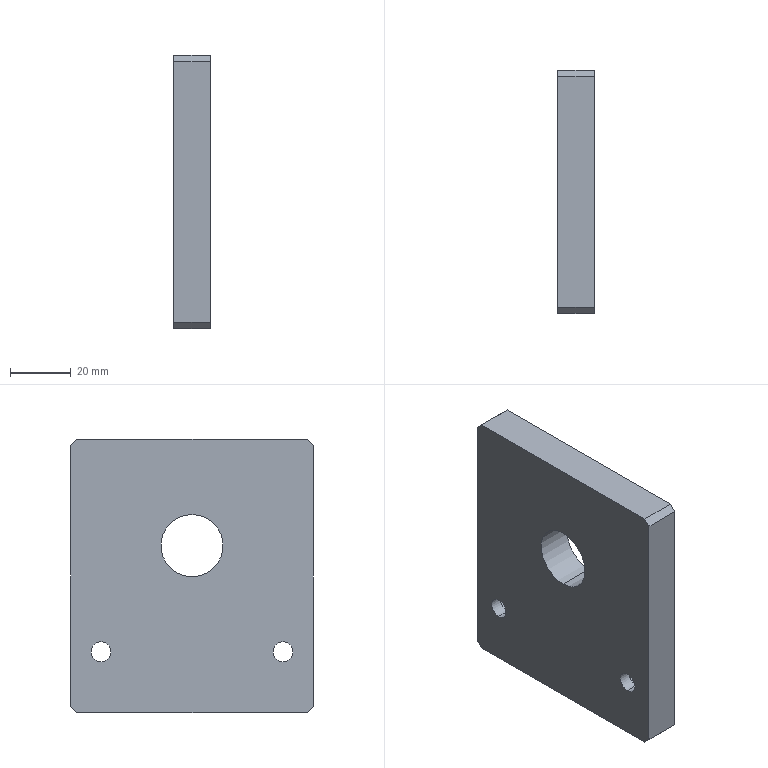Part | SolidWorks | features BaseBody 1 | 1 solid | 22 faces | box 12 x 80 x 90 mm | volume 80549 mm3 | plane 12 | cylinder 10 | commonest cylinder face diameters 6.6 x4 11 x4 20.5 x2
STEP:
#1=CARTESIAN_POINT('',(12.,40.,-45.25));
#2=VERTEX_POINT('',#1);
#3=CARTESIAN_POINT('',(12.,40.,-24.75));
#4=VERTEX_POINT('',#3);
#5=CARTESIAN_POINT('',(12.,40.,-35.));
#6=DIRECTION('',(-1.,0.,0.));
#7=DIRECTION('',(0.,0.,1.));
#8=AXIS2_PLACEMENT_3D('',#5,#6,#7);
#9=CIRCLE('',#8,10.25);
#10=EDGE_CURVE('',#2,#4,#9,.T.);
#11=ORIENTED_EDGE('',*,*,#10,.F.);
#12=CARTESIAN_POINT('',(0.,40.,-45.25));
#13=VERTEX_POINT('',#12);
#14=CARTESIAN_POINT('',(0.,40.,-45.25));
#15=DIRECTION('',(-1.,0.,0.));
#16=VECTOR('',#15,1000.);
#17=LINE('',#14,#16);
#18=EDGE_CURVE('',#2,#13,#17,.T.);
#19=ORIENTED_EDGE('',*,*,#18,.T.);
#20=CARTESIAN_POINT('',(0.,40.,-24.75));
#21=VERTEX_POINT('',#20);
#22=CARTESIAN_POINT('',(0.,40.,-35.));
#23=DIRECTION('',(1.,0.,0.));
#24=DIRECTION('',(0.,0.,1.));
#25=AXIS2_PLACEMENT_3D('',#22,#23,#24);
#26=CIRCLE('',#25,10.25);
#27=EDGE_CURVE('',#21,#13,#26,.T.);
#28=ORIENTED_EDGE('',*,*,#27,.F.);
#29=CARTESIAN_POINT('',(0.,40.,-24.75));
#30=DIRECTION('',(-1.,0.,0.));
#31=VECTOR('',#30,1000.);
#32=LINE('',#29,#31);
#33=EDGE_CURVE('',#4,#21,#32,.T.);
#34=ORIENTED_EDGE('',*,*,#33,.F.);
#35=EDGE_LOOP('',(#11,#19,#28,#34));
#36=FACE_OUTER_BOUND('',#35,.T.);
#37=CARTESIAN_POINT('',(0.,40.,-35.));
#38=DIRECTION('',(-1.,0.,0.));
#39=DIRECTION('',(0.,0.,1.));
#40=AXIS2_PLACEMENT_3D('',#37,#38,#39);
#41=CYLINDRICAL_SURFACE('',#40,10.25);
#42=ADVANCED_FACE('',(#36),#41,.F.);
#43=CARTESIAN_POINT('',(0.,10.,-66.7));
#44=VERTEX_POINT('',#43);
#45=CARTESIAN_POINT('',(0.,10.,-73.3));
#46=VERTEX_POINT('',#45);
#47=CARTESIAN_POINT('',(0.,10.,-70.));
#48=DIRECTION('',(1.,0.,0.));
#49=DIRECTION('',(0.,0.,-1.));
#50=AXIS2_PLACEMENT_3D('',#47,#48,#49);
#51=CIRCLE('',#50,3.3);
#52=EDGE_CURVE('',#44,#46,#51,.T.);
#53=ORIENTED_EDGE('',*,*,#52,.F.);
#54=CARTESIAN_POINT('',(4.,10.,-66.7));
#55=VERTEX_POINT('',#54);
#56=CARTESIAN_POINT('',(12.,10.,-66.7));
#57=DIRECTION('',(1.,0.,0.));
#58=VECTOR('',#57,1000.);
#59=LINE('',#56,#58);
#60=EDGE_CURVE('',#44,#55,#59,.T.);
#61=ORIENTED_EDGE('',*,*,#60,.T.);
#62=CARTESIAN_POINT('',(4.,10.,-73.3));
#63=VERTEX_POINT('',#62);
#64=CARTESIAN_POINT('',(4.,10.,-70.));
#65=DIRECTION('',(-1.,0.,0.));
#66=DIRECTION('',(0.,0.,-1.));
#67=AXIS2_PLACEMENT_3D('',#64,#65,#66);
#68=CIRCLE('',#67,3.3);
#69=EDGE_CURVE('',#63,#55,#68,.T.);
#70=ORIENTED_EDGE('',*,*,#69,.F.);
#71=CARTESIAN_POINT('',(12.,10.,-73.3));
#72=DIRECTION('',(1.,0.,0.));
#73=VECTOR('',#72,1000.);
#74=LINE('',#71,#73);
#75=EDGE_CURVE('',#46,#63,#74,.T.);
#76=ORIENTED_EDGE('',*,*,#75,.F.);
#77=EDGE_LOOP('',(#53,#61,#70,#76));
#78=FACE_OUTER_BOUND('',#77,.T.);
#79=CARTESIAN_POINT('',(12.,10.,-70.));
#80=DIRECTION('',(1.,0.,0.));
#81=DIRECTION('',(0.,0.,-1.));
#82=AXIS2_PLACEMENT_3D('',#79,#80,#81);
#83=CYLINDRICAL_SURFACE('',#82,3.3);
#84=ADVANCED_FACE('',(#78),#83,.F.);
#85=CARTESIAN_POINT('',(0.,70.,-66.7));
#86=VERTEX_POINT('',#85);
#87=CARTESIAN_POINT('',(0.,70.,-73.3));
#88=VERTEX_POINT('',#87);
#89=CARTESIAN_POINT('',(0.,70.,-70.));
#90=DIRECTION('',(1.,0.,0.));
#91=DIRECTION('',(0.,0.,-1.));
#92=AXIS2_PLACEMENT_3D('',#89,#90,#91);
#93=CIRCLE('',#92,3.3);
#94=EDGE_CURVE('',#86,#88,#93,.T.);
#95=ORIENTED_EDGE('',*,*,#94,.F.);
#96=CARTESIAN_POINT('',(4.,70.,-66.7));
#97=VERTEX_POINT('',#96);
#98=CARTESIAN_POINT('',(12.,70.,-66.7));
#99=DIRECTION('',(1.,0.,0.));
#100=VECTOR('',#99,1000.);
#101=LINE('',#98,#100);
#102=EDGE_CURVE('',#86,#97,#101,.T.);
#103=ORIENTED_EDGE('',*,*,#102,.T.);
#104=CARTESIAN_POINT('',(4.,70.,-73.3));
#105=VERTEX_POINT('',#104);
#106=CARTESIAN_POINT('',(4.,70.,-70.));
#107=DIRECTION('',(-1.,0.,0.));
#108=DIRECTION('',(0.,0.,-1.));
#109=AXIS2_PLACEMENT_3D('',#106,#107,#108);
#110=CIRCLE('',#109,3.3);
#111=EDGE_CURVE('',#105,#97,#110,.T.);
#112=ORIENTED_EDGE('',*,*,#111,.F.);
#113=CARTESIAN_POINT('',(12.,70.,-73.3));
#114=DIRECTION('',(1.,0.,0.));
#115=VECTOR('',#114,1000.);
#116=LINE('',#113,#115);
#117=EDGE_CURVE('',#88,#105,#116,.T.);
#118=ORIENTED_EDGE('',*,*,#117,.F.);
#119=EDGE_LOOP('',(#95,#103,#112,#118));
#120=FACE_OUTER_BOUND('',#119,.T.);
#121=CARTESIAN_POINT('',(12.,70.,-70.));
#122=DIRECTION('',(1.,0.,0.));
#123=DIRECTION('',(0.,0.,-1.));
#124=AXIS2_PLACEMENT_3D('',#121,#122,#123);
#125=CYLINDRICAL_SURFACE('',#124,3.3);
#126=ADVANCED_FACE('',(#120),#125,.F.);
#127=CARTESIAN_POINT('',(4.,10.,-75.5));
#128=VERTEX_POINT('',#127);
#129=CARTESIAN_POINT('',(4.,10.,-64.5));
#130=VERTEX_POINT('',#129);
#131=CARTESIAN_POINT('',(4.,10.,-70.));
#132=DIRECTION('',(-1.,0.,0.));
#133=DIRECTION('',(0.,0.,-1.));
#134=AXIS2_PLACEMENT_3D('',#131,#132,#133);
#135=CIRCLE('',#134,5.5);
#136=EDGE_CURVE('',#128,#130,#135,.T.);
#137=ORIENTED_EDGE('',*,*,#136,.T.);
#138=CARTESIAN_POINT('',(12.,10.,-64.5));
#139=VERTEX_POINT('',#138);
#140=CARTESIAN_POINT('',(12.,10.,-64.5));
#141=DIRECTION('',(1.,0.,0.));
#142=VECTOR('',#141,1000.);
#143=LINE('',#140,#142);
#144=EDGE_CURVE('',#130,#139,#143,.T.);
#145=ORIENTED_EDGE('',*,*,#144,.T.);
#146=CARTESIAN_POINT('',(12.,10.,-75.5));
#147=VERTEX_POINT('',#146);
#148=CARTESIAN_POINT('',(12.,10.,-70.));
#149=DIRECTION('',(1.,0.,0.));
#150=DIRECTION('',(0.,0.,-1.));
#151=AXIS2_PLACEMENT_3D('',#148,#149,#150);
#152=CIRCLE('',#151,5.5);
#153=EDGE_CURVE('',#139,#147,#152,.T.);
#154=ORIENTED_EDGE('',*,*,#153,.T.);
#155=CARTESIAN_POINT('',(12.,10.,-75.5));
#156=DIRECTION('',(1.,0.,0.));
#157=VECTOR('',#156,1000.);
#158=LINE('',#155,#157);
#159=EDGE_CURVE('',#128,#147,#158,.T.);
#160=ORIENTED_EDGE('',*,*,#159,.F.);
#161=EDGE_LOOP('',(#137,#145,#154,#160));
#162=FACE_OUTER_BOUND('',#161,.T.);
#163=CARTESIAN_POINT('',(12.,10.,-70.));
#164=DIRECTION('',(1.,0.,0.));
#165=DIRECTION('',(0.,0.,-1.));
#166=AXIS2_PLACEMENT_3D('',#163,#164,#165);
#167=CYLINDRICAL_SURFACE('',#166,5.5);
#168=ADVANCED_FACE('',(#162),#167,.F.);
#169=CARTESIAN_POINT('',(4.,70.,-75.5));
#170=VERTEX_POINT('',#169);
#171=CARTESIAN_POINT('',(4.,70.,-64.5));
#172=VERTEX_POINT('',#171);
#173=CARTESIAN_POINT('',(4.,70.,-70.));
#174=DIRECTION('',(-1.,0.,0.));
#175=DIRECTION('',(0.,0.,-1.));
#176=AXIS2_PLACEMENT_3D('',#173,#174,#175);
#177=CIRCLE('',#176,5.5);
#178=EDGE_CURVE('',#170,#172,#177,.T.);
#179=ORIENTED_EDGE('',*,*,#178,.T.);
#180=CARTESIAN_POINT('',(12.,70.,-64.5));
#181=VERTEX_POINT('',#180);
#182=CARTESIAN_POINT('',(12.,70.,-64.5));
#183=DIRECTION('',(1.,0.,0.));
#184=VECTOR('',#183,1000.);
#185=LINE('',#182,#184);
#186=EDGE_CURVE('',#172,#181,#185,.T.);
#187=ORIENTED_EDGE('',*,*,#186,.T.);
#188=CARTESIAN_POINT('',(12.,70.,-75.5));
#189=VERTEX_POINT('',#188);
#190=CARTESIAN_POINT('',(12.,70.,-70.));
#191=DIRECTION('',(1.,0.,0.));
#192=DIRECTION('',(0.,0.,-1.));
#193=AXIS2_PLACEMENT_3D('',#190,#191,#192);
#194=CIRCLE('',#193,5.5);
#195=EDGE_CURVE('',#181,#189,#194,.T.);
#196=ORIENTED_EDGE('',*,*,#195,.T.);
#197=CARTESIAN_POINT('',(12.,70.,-75.5));
#198=DIRECTION('',(1.,0.,0.));
#199=VECTOR('',#198,1000.);
#200=LINE('',#197,#199);
#201=EDGE_CURVE('',#170,#189,#200,.T.);
#202=ORIENTED_EDGE('',*,*,#201,.F.);
#203=EDGE_LOOP('',(#179,#187,#196,#202));
#204=FACE_OUTER_BOUND('',#203,.T.);
#205=CARTESIAN_POINT('',(12.,70.,-70.));
#206=DIRECTION('',(1.,0.,0.));
#207=DIRECTION('',(0.,0.,-1.));
#208=AXIS2_PLACEMENT_3D('',#205,#206,#207);
#209=CYLINDRICAL_SURFACE('',#208,5.5);
#210=ADVANCED_FACE('',(#204),#209,.F.);
#211=CARTESIAN_POINT('',(0.,2.,0.));
#212=VERTEX_POINT('',#211);
#213=CARTESIAN_POINT('',(0.,78.,0.));
#214=VERTEX_POINT('',#213);
#215=CARTESIAN_POINT('',(0.,0.,0.));
#216=DIRECTION('',(0.,1.,0.));
#217=VECTOR('',#216,1000.);
#218=LINE('',#215,#217);
#219=EDGE_CURVE('',#212,#214,#218,.T.);
#220=ORIENTED_EDGE('',*,*,#219,.T.);
#221=CARTESIAN_POINT('',(0.,80.,-2.));
#222=VERTEX_POINT('',#221);
#223=CARTESIAN_POINT('',(0.,78.,0.));
#224=DIRECTION('',(0.,0.7071,-0.7071));
#225=VECTOR('',#224,1000.);
#226=LINE('',#223,#225);
#227=EDGE_CURVE('',#214,#222,#226,.T.);
#228=ORIENTED_EDGE('',*,*,#227,.T.);
#229=CARTESIAN_POINT('',(0.,80.,-88.));
#230=VERTEX_POINT('',#229);
#231=CARTESIAN_POINT('',(0.,80.,0.));
#232=DIRECTION('',(0.,0.,-1.));
#233=VECTOR('',#232,1000.);
#234=LINE('',#231,#233);
#235=EDGE_CURVE('',#222,#230,#234,.T.);
#236=ORIENTED_EDGE('',*,*,#235,.T.);
#237=CARTESIAN_POINT('',(0.,78.,-90.));
#238=VERTEX_POINT('',#237);
#239=CARTESIAN_POINT('',(0.,80.,-88.));
#240=DIRECTION('',(0.,-0.7071,-0.7071));
#241=VECTOR('',#240,1000.);
#242=LINE('',#239,#241);
#243=EDGE_CURVE('',#230,#238,#242,.T.);
#244=ORIENTED_EDGE('',*,*,#243,.T.);
#245=CARTESIAN_POINT('',(0.,2.,-90.));
#246=VERTEX_POINT('',#245);
#247=CARTESIAN_POINT('',(0.,0.,-90.));
#248=DIRECTION('',(0.,-1.,0.));
#249=VECTOR('',#248,1000.);
#250=LINE('',#247,#249);
#251=EDGE_CURVE('',#238,#246,#250,.T.);
#252=ORIENTED_EDGE('',*,*,#251,.T.);
#253=CARTESIAN_POINT('',(0.,0.,-88.));
#254=VERTEX_POINT('',#253);
#255=CARTESIAN_POINT('',(0.,2.,-90.));
#256=DIRECTION('',(0.,-0.7071,0.7071));
#257=VECTOR('',#256,1000.);
#258=LINE('',#255,#257);
#259=EDGE_CURVE('',#246,#254,#258,.T.);
#260=ORIENTED_EDGE('',*,*,#259,.T.);
#261=CARTESIAN_POINT('',(0.,0.,-2.));
#262=VERTEX_POINT('',#261);
#263=CARTESIAN_POINT('',(0.,0.,0.));
#264=DIRECTION('',(0.,0.,1.));
#265=VECTOR('',#264,1000.);
#266=LINE('',#263,#265);
#267=EDGE_CURVE('',#254,#262,#266,.T.);
#268=ORIENTED_EDGE('',*,*,#267,.T.);
#269=CARTESIAN_POINT('',(0.,0.,-2.));
#270=DIRECTION('',(0.,0.7071,0.7071));
#271=VECTOR('',#270,1000.);
#272=LINE('',#269,#271);
#273=EDGE_CURVE('',#262,#212,#272,.T.);
#274=ORIENTED_EDGE('',*,*,#273,.T.);
#275=EDGE_LOOP('',(#220,#228,#236,#244,#252,#260,#268,#274));
#276=FACE_OUTER_BOUND('',#275,.T.);
#277=ORIENTED_EDGE('',*,*,#27,.T.);
#278=CARTESIAN_POINT('',(0.,40.,-35.));
#279=DIRECTION('',(1.,0.,0.));
#280=DIRECTION('',(0.,0.,1.));
#281=AXIS2_PLACEMENT_3D('',#278,#279,#280);
#282=CIRCLE('',#281,10.25);
#283=EDGE_CURVE('',#13,#21,#282,.T.);
#284=ORIENTED_EDGE('',*,*,#283,.T.);
#285=EDGE_LOOP('',(#277,#284));
#286=FACE_BOUND('',#285,.T.);
#287=CARTESIAN_POINT('',(0.,10.,-70.));
#288=DIRECTION('',(1.,0.,0.));
#289=DIRECTION('',(0.,0.,-1.));
#290=AXIS2_PLACEMENT_3D('',#287,#288,#289);
#291=CIRCLE('',#290,3.3);
#292=EDGE_CURVE('',#46,#44,#291,.T.);
#293=ORIENTED_EDGE('',*,*,#292,.T.);
#294=ORIENTED_EDGE('',*,*,#52,.T.);
#295=EDGE_LOOP('',(#293,#294));
#296=FACE_BOUND('',#295,.T.);
#297=CARTESIAN_POINT('',(0.,70.,-70.));
#298=DIRECTION('',(1.,0.,0.));
#299=DIRECTION('',(0.,0.,-1.));
#300=AXIS2_PLACEMENT_3D('',#297,#298,#299);
#301=CIRCLE('',#300,3.3);
#302=EDGE_CURVE('',#88,#86,#301,.T.);
#303=ORIENTED_EDGE('',*,*,#302,.T.);
#304=ORIENTED_EDGE('',*,*,#94,.T.);
#305=EDGE_LOOP('',(#303,#304));
#306=FACE_BOUND('',#305,.T.);
#307=CARTESIAN_POINT('',(0.,0.,0.));
#308=DIRECTION('',(-1.,0.,0.));
#309=DIRECTION('',(0.,0.,1.));
#310=AXIS2_PLACEMENT_3D('',#307,#308,#309);
#311=PLANE('',#310);
#312=ADVANCED_FACE('',(#276,#286,#296,#306),#311,.T.);
#313=CARTESIAN_POINT('',(12.,80.,-2.));
#314=VERTEX_POINT('',#313);
#315=CARTESIAN_POINT('',(12.,80.,-2.));
#316=DIRECTION('',(1.,0.,0.));
#317=VECTOR('',#316,1000.);
#318=LINE('',#315,#317);
#319=EDGE_CURVE('',#222,#314,#318,.T.);
#320=ORIENTED_EDGE('',*,*,#319,.F.);
#321=ORIENTED_EDGE('',*,*,#227,.F.);
#322=CARTESIAN_POINT('',(12.,78.,0.));
#323=VERTEX_POINT('',#322);
#324=CARTESIAN_POINT('',(12.,78.,0.));
#325=DIRECTION('',(-1.,0.,0.));
#326=VECTOR('',#325,1000.);
#327=LINE('',#324,#326);
#328=EDGE_CURVE('',#323,#214,#327,.T.);
#329=ORIENTED_EDGE('',*,*,#328,.F.);
#330=CARTESIAN_POINT('',(12.,78.,0.));
#331=DIRECTION('',(0.,-0.7071,0.7071));
#332=VECTOR('',#331,1000.);
#333=LINE('',#330,#332);
#334=EDGE_CURVE('',#314,#323,#333,.T.);
#335=ORIENTED_EDGE('',*,*,#334,.F.);
#336=EDGE_LOOP('',(#320,#321,#329,#335));
#337=FACE_OUTER_BOUND('',#336,.T.);
#338=CARTESIAN_POINT('',(12.,78.,0.));
#339=DIRECTION('',(0.,-0.7071,-0.7071));
#340=DIRECTION('',(0.,0.7071,-0.7071));
#341=AXIS2_PLACEMENT_3D('',#338,#339,#340);
#342=PLANE('',#341);
#343=ADVANCED_FACE('',(#337),#342,.F.);
#344=ORIENTED_EDGE('',*,*,#328,.T.);
#345=ORIENTED_EDGE('',*,*,#219,.F.);
#346=CARTESIAN_POINT('',(12.,2.,0.));
#347=VERTEX_POINT('',#346);
#348=CARTESIAN_POINT('',(12.,2.,0.));
#349=DIRECTION('',(-1.,0.,0.));
#350=VECTOR('',#349,1000.);
#351=LINE('',#348,#350);
#352=EDGE_CURVE('',#347,#212,#351,.T.);
#353=ORIENTED_EDGE('',*,*,#352,.F.);
#354=CARTESIAN_POINT('',(12.,0.,0.));
#355=DIRECTION('',(0.,-1.,0.));
#356=VECTOR('',#355,1000.);
#357=LINE('',#354,#356);
#358=EDGE_CURVE('',#323,#347,#357,.T.);
#359=ORIENTED_EDGE('',*,*,#358,.F.);
#360=EDGE_LOOP('',(#344,#345,#353,#359));
#361=FACE_OUTER_BOUND('',#360,.T.);
#362=CARTESIAN_POINT('',(12.,0.,0.));
#363=DIRECTION('',(0.,0.,-1.));
#364=DIRECTION('',(-1.,0.,0.));
#365=AXIS2_PLACEMENT_3D('',#362,#363,#364);
#366=PLANE('',#365);
#367=ADVANCED_FACE('',(#361),#366,.F.);
#368=ORIENTED_EDGE('',*,*,#352,.T.);
#369=ORIENTED_EDGE('',*,*,#273,.F.);
#370=CARTESIAN_POINT('',(12.,0.,-2.));
#371=VERTEX_POINT('',#370);
#372=CARTESIAN_POINT('',(12.,0.,-2.));
#373=DIRECTION('',(-1.,0.,0.));
#374=VECTOR('',#373,1000.);
#375=LINE('',#372,#374);
#376=EDGE_CURVE('',#371,#262,#375,.T.);
#377=ORIENTED_EDGE('',*,*,#376,.F.);
#378=CARTESIAN_POINT('',(12.,0.,-2.));
#379=DIRECTION('',(0.,-0.7071,-0.7071));
#380=VECTOR('',#379,1000.);
#381=LINE('',#378,#380);
#382=EDGE_CURVE('',#347,#371,#381,.T.);
#383=ORIENTED_EDGE('',*,*,#382,.F.);
#384=EDGE_LOOP('',(#368,#369,#377,#383));
#385=FACE_OUTER_BOUND('',#384,.T.);
#386=CARTESIAN_POINT('',(12.,0.,-2.));
#387=DIRECTION('',(0.,0.7071,-0.7071));
#388=DIRECTION('',(0.,0.7071,0.7071));
#389=AXIS2_PLACEMENT_3D('',#386,#387,#388);
#390=PLANE('',#389);
#391=ADVANCED_FACE('',(#385),#390,.F.);
#392=ORIENTED_EDGE('',*,*,#376,.T.);
#393=ORIENTED_EDGE('',*,*,#267,.F.);
#394=CARTESIAN_POINT('',(12.,0.,-88.));
#395=VERTEX_POINT('',#394);
#396=CARTESIAN_POINT('',(12.,0.,-88.));
#397=DIRECTION('',(-1.,0.,0.));
#398=VECTOR('',#397,1000.);
#399=LINE('',#396,#398);
#400=EDGE_CURVE('',#395,#254,#399,.T.);
#401=ORIENTED_EDGE('',*,*,#400,.F.);
#402=CARTESIAN_POINT('',(12.,0.,0.));
#403=DIRECTION('',(0.,0.,-1.));
#404=VECTOR('',#403,1000.);
#405=LINE('',#402,#404);
#406=EDGE_CURVE('',#371,#395,#405,.T.);
#407=ORIENTED_EDGE('',*,*,#406,.F.);
#408=EDGE_LOOP('',(#392,#393,#401,#407));
#409=FACE_OUTER_BOUND('',#408,.T.);
#410=CARTESIAN_POINT('',(12.,0.,0.));
#411=DIRECTION('',(0.,1.,0.));
#412=DIRECTION('',(0.,0.,1.));
#413=AXIS2_PLACEMENT_3D('',#410,#411,#412);
#414=PLANE('',#413);
#415=ADVANCED_FACE('',(#409),#414,.F.);
#416=ORIENTED_EDGE('',*,*,#400,.T.);
#417=ORIENTED_EDGE('',*,*,#259,.F.);
#418=CARTESIAN_POINT('',(12.,2.,-90.));
#419=VERTEX_POINT('',#418);
#420=CARTESIAN_POINT('',(12.,2.,-90.));
#421=DIRECTION('',(-1.,0.,0.));
#422=VECTOR('',#421,1000.);
#423=LINE('',#420,#422);
#424=EDGE_CURVE('',#419,#246,#423,.T.);
#425=ORIENTED_EDGE('',*,*,#424,.F.);
#426=CARTESIAN_POINT('',(12.,2.,-90.));
#427=DIRECTION('',(0.,0.7071,-0.7071));
#428=VECTOR('',#427,1000.);
#429=LINE('',#426,#428);
#430=EDGE_CURVE('',#395,#419,#429,.T.);
#431=ORIENTED_EDGE('',*,*,#430,.F.);
#432=EDGE_LOOP('',(#416,#417,#425,#431));
#433=FACE_OUTER_BOUND('',#432,.T.);
#434=CARTESIAN_POINT('',(12.,2.,-90.));
#435=DIRECTION('',(0.,0.7071,0.7071));
#436=DIRECTION('',(0.,-0.7071,0.7071));
#437=AXIS2_PLACEMENT_3D('',#434,#435,#436);
#438=PLANE('',#437);
#439=ADVANCED_FACE('',(#433),#438,.F.);
#440=CARTESIAN_POINT('',(12.,78.,-90.));
#441=VERTEX_POINT('',#440);
#442=CARTESIAN_POINT('',(12.,78.,-90.));
#443=DIRECTION('',(-1.,0.,0.));
#444=VECTOR('',#443,1000.);
#445=LINE('',#442,#444);
#446=EDGE_CURVE('',#441,#238,#445,.T.);
#447=ORIENTED_EDGE('',*,*,#446,.F.);
#448=CARTESIAN_POINT('',(12.,0.,-90.));
#449=DIRECTION('',(0.,1.,0.));
#450=VECTOR('',#449,1000.);
#451=LINE('',#448,#450);
#452=EDGE_CURVE('',#419,#441,#451,.T.);
#453=ORIENTED_EDGE('',*,*,#452,.F.);
#454=ORIENTED_EDGE('',*,*,#424,.T.);
#455=ORIENTED_EDGE('',*,*,#251,.F.);
#456=EDGE_LOOP('',(#447,#453,#454,#455));
#457=FACE_OUTER_BOUND('',#456,.T.);
#458=CARTESIAN_POINT('',(12.,0.,-90.));
#459=DIRECTION('',(0.,0.,1.));
#460=DIRECTION('',(1.,0.,0.));
#461=AXIS2_PLACEMENT_3D('',#458,#459,#460);
#462=PLANE('',#461);
#463=ADVANCED_FACE('',(#457),#462,.F.);
#464=ORIENTED_EDGE('',*,*,#446,.T.);
#465=ORIENTED_EDGE('',*,*,#243,.F.);
#466=CARTESIAN_POINT('',(12.,80.,-88.));
#467=VERTEX_POINT('',#466);
#468=CARTESIAN_POINT('',(12.,80.,-88.));
#469=DIRECTION('',(-1.,0.,0.));
#470=VECTOR('',#469,1000.);
#471=LINE('',#468,#470);
#472=EDGE_CURVE('',#467,#230,#471,.T.);
#473=ORIENTED_EDGE('',*,*,#472,.F.);
#474=CARTESIAN_POINT('',(12.,80.,-88.));
#475=DIRECTION('',(0.,0.7071,0.7071));
#476=VECTOR('',#475,1000.);
#477=LINE('',#474,#476);
#478=EDGE_CURVE('',#441,#467,#477,.T.);
#479=ORIENTED_EDGE('',*,*,#478,.F.);
#480=EDGE_LOOP('',(#464,#465,#473,#479));
#481=FACE_OUTER_BOUND('',#480,.T.);
#482=CARTESIAN_POINT('',(12.,80.,-88.));
#483=DIRECTION('',(0.,-0.7071,0.7071));
#484=DIRECTION('',(0.,-0.7071,-0.7071));
#485=AXIS2_PLACEMENT_3D('',#482,#483,#484);
#486=PLANE('',#485);
#487=ADVANCED_FACE('',(#481),#486,.F.);
#488=ORIENTED_EDGE('',*,*,#472,.T.);
#489=ORIENTED_EDGE('',*,*,#235,.F.);
#490=ORIENTED_EDGE('',*,*,#319,.T.);
#491=CARTESIAN_POINT('',(12.,80.,0.));
#492=DIRECTION('',(0.,0.,1.));
#493=VECTOR('',#492,1000.);
#494=LINE('',#491,#493);
#495=EDGE_CURVE('',#467,#314,#494,.T.);
#496=ORIENTED_EDGE('',*,*,#495,.F.);
#497=EDGE_LOOP('',(#488,#489,#490,#496));
#498=FACE_OUTER_BOUND('',#497,.T.);
#499=CARTESIAN_POINT('',(12.,80.,0.));
#500=DIRECTION('',(0.,-1.,0.));
#501=DIRECTION('',(0.,0.,-1.));
#502=AXIS2_PLACEMENT_3D('',#499,#500,#501);
#503=PLANE('',#502);
#504=ADVANCED_FACE('',(#498),#503,.F.);
#505=ORIENTED_EDGE('',*,*,#18,.F.);
#506=CARTESIAN_POINT('',(12.,40.,-35.));
#507=DIRECTION('',(-1.,0.,0.));
#508=DIRECTION('',(0.,0.,1.));
#509=AXIS2_PLACEMENT_3D('',#506,#507,#508);
#510=CIRCLE('',#509,10.25);
#511=EDGE_CURVE('',#4,#2,#510,.T.);
#512=ORIENTED_EDGE('',*,*,#511,.F.);
#513=ORIENTED_EDGE('',*,*,#33,.T.);
#514=ORIENTED_EDGE('',*,*,#283,.F.);
#515=EDGE_LOOP('',(#505,#512,#513,#514));
#516=FACE_OUTER_BOUND('',#515,.T.);
#517=CARTESIAN_POINT('',(0.,40.,-35.));
#518=DIRECTION('',(-1.,0.,0.));
#519=DIRECTION('',(0.,0.,1.));
#520=AXIS2_PLACEMENT_3D('',#517,#518,#519);
#521=CYLINDRICAL_SURFACE('',#520,10.25);
#522=ADVANCED_FACE('',(#516),#521,.F.);
#523=ORIENTED_EDGE('',*,*,#60,.F.);
#524=ORIENTED_EDGE('',*,*,#292,.F.);
#525=ORIENTED_EDGE('',*,*,#75,.T.);
#526=CARTESIAN_POINT('',(4.,10.,-70.));
#527=DIRECTION('',(-1.,0.,0.));
#528=DIRECTION('',(0.,0.,-1.));
#529=AXIS2_PLACEMENT_3D('',#526,#527,#528);
#530=CIRCLE('',#529,3.3);
#531=EDGE_CURVE('',#55,#63,#530,.T.);
#532=ORIENTED_EDGE('',*,*,#531,.F.);
#533=EDGE_LOOP('',(#523,#524,#525,#532));
#534=FACE_OUTER_BOUND('',#533,.T.);
#535=CARTESIAN_POINT('',(12.,10.,-70.));
#536=DIRECTION('',(1.,0.,0.));
#537=DIRECTION('',(0.,0.,-1.));
#538=AXIS2_PLACEMENT_3D('',#535,#536,#537);
#539=CYLINDRICAL_SURFACE('',#538,3.3);
#540=ADVANCED_FACE('',(#534),#539,.F.);
#541=ORIENTED_EDGE('',*,*,#102,.F.);
#542=ORIENTED_EDGE('',*,*,#302,.F.);
#543=ORIENTED_EDGE('',*,*,#117,.T.);
#544=CARTESIAN_POINT('',(4.,70.,-70.));
#545=DIRECTION('',(-1.,0.,0.));
#546=DIRECTION('',(0.,0.,-1.));
#547=AXIS2_PLACEMENT_3D('',#544,#545,#546);
#548=CIRCLE('',#547,3.3);
#549=EDGE_CURVE('',#97,#105,#548,.T.);
#550=ORIENTED_EDGE('',*,*,#549,.F.);
#551=EDGE_LOOP('',(#541,#542,#543,#550));
#552=FACE_OUTER_BOUND('',#551,.T.);
#553=CARTESIAN_POINT('',(12.,70.,-70.));
#554=DIRECTION('',(1.,0.,0.));
#555=DIRECTION('',(0.,0.,-1.));
#556=AXIS2_PLACEMENT_3D('',#553,#554,#555);
#557=CYLINDRICAL_SURFACE('',#556,3.3);
#558=ADVANCED_FACE('',(#552),#557,.F.);
#559=ORIENTED_EDGE('',*,*,#478,.T.);
#560=ORIENTED_EDGE('',*,*,#495,.T.);
#561=ORIENTED_EDGE('',*,*,#334,.T.);
#562=ORIENTED_EDGE('',*,*,#358,.T.);
#563=ORIENTED_EDGE('',*,*,#382,.T.);
#564=ORIENTED_EDGE('',*,*,#406,.T.);
#565=ORIENTED_EDGE('',*,*,#430,.T.);
#566=ORIENTED_EDGE('',*,*,#452,.T.);
#567=EDGE_LOOP('',(#559,#560,#561,#562,#563,#564,#565,#566));
#568=FACE_OUTER_BOUND('',#567,.T.);
#569=ORIENTED_EDGE('',*,*,#511,.T.);
#570=ORIENTED_EDGE('',*,*,#10,.T.);
#571=EDGE_LOOP('',(#569,#570));
#572=FACE_BOUND('',#571,.T.);
#573=CARTESIAN_POINT('',(12.,10.,-70.));
#574=DIRECTION('',(1.,0.,0.));
#575=DIRECTION('',(0.,0.,-1.));
#576=AXIS2_PLACEMENT_3D('',#573,#574,#575);
#577=CIRCLE('',#576,5.5);
#578=EDGE_CURVE('',#147,#139,#577,.T.);
#579=ORIENTED_EDGE('',*,*,#578,.F.);
#580=ORIENTED_EDGE('',*,*,#153,.F.);
#581=EDGE_LOOP('',(#579,#580));
#582=FACE_BOUND('',#581,.T.);
#583=CARTESIAN_POINT('',(12.,70.,-70.));
#584=DIRECTION('',(1.,0.,0.));
#585=DIRECTION('',(0.,0.,-1.));
#586=AXIS2_PLACEMENT_3D('',#583,#584,#585);
#587=CIRCLE('',#586,5.5);
#588=EDGE_CURVE('',#189,#181,#587,.T.);
#589=ORIENTED_EDGE('',*,*,#588,.F.);
#590=ORIENTED_EDGE('',*,*,#195,.F.);
#591=EDGE_LOOP('',(#589,#590));
#592=FACE_BOUND('',#591,.T.);
#593=CARTESIAN_POINT('',(12.,0.,0.));
#594=DIRECTION('',(-1.,0.,0.));
#595=DIRECTION('',(0.,0.,1.));
#596=AXIS2_PLACEMENT_3D('',#593,#594,#595);
#597=PLANE('',#596);
#598=ADVANCED_FACE('',(#568,#572,#582,#592),#597,.F.);
#599=ORIENTED_EDGE('',*,*,#136,.F.);
#600=CARTESIAN_POINT('',(4.,10.,-70.));
#601=DIRECTION('',(-1.,0.,0.));
#602=DIRECTION('',(0.,0.,-1.));
#603=AXIS2_PLACEMENT_3D('',#600,#601,#602);
#604=CIRCLE('',#603,5.5);
#605=EDGE_CURVE('',#130,#128,#604,.T.);
#606=ORIENTED_EDGE('',*,*,#605,.F.);
#607=EDGE_LOOP('',(#599,#606));
#608=FACE_OUTER_BOUND('',#607,.T.);
#609=ORIENTED_EDGE('',*,*,#69,.T.);
#610=ORIENTED_EDGE('',*,*,#531,.T.);
#611=EDGE_LOOP('',(#609,#610));
#612=FACE_BOUND('',#611,.T.);
#613=CARTESIAN_POINT('',(4.,13.3,-70.));
#614=DIRECTION('',(-1.,0.,0.));
#615=DIRECTION('',(0.,0.,1.));
#616=AXIS2_PLACEMENT_3D('',#613,#614,#615);
#617=PLANE('',#616);
#618=ADVANCED_FACE('',(#608,#612),#617,.F.);
#619=ORIENTED_EDGE('',*,*,#178,.F.);
#620=CARTESIAN_POINT('',(4.,70.,-70.));
#621=DIRECTION('',(-1.,0.,0.));
#622=DIRECTION('',(0.,0.,-1.));
#623=AXIS2_PLACEMENT_3D('',#620,#621,#622);
#624=CIRCLE('',#623,5.5);
#625=EDGE_CURVE('',#172,#170,#624,.T.);
#626=ORIENTED_EDGE('',*,*,#625,.F.);
#627=EDGE_LOOP('',(#619,#626));
#628=FACE_OUTER_BOUND('',#627,.T.);
#629=ORIENTED_EDGE('',*,*,#111,.T.);
#630=ORIENTED_EDGE('',*,*,#549,.T.);
#631=EDGE_LOOP('',(#629,#630));
#632=FACE_BOUND('',#631,.T.);
#633=CARTESIAN_POINT('',(4.,73.3,-70.));
#634=DIRECTION('',(-1.,0.,0.));
#635=DIRECTION('',(0.,0.,1.));
#636=AXIS2_PLACEMENT_3D('',#633,#634,#635);
#637=PLANE('',#636);
#638=ADVANCED_FACE('',(#628,#632),#637,.F.);
#639=ORIENTED_EDGE('',*,*,#144,.F.);
#640=ORIENTED_EDGE('',*,*,#605,.T.);
#641=ORIENTED_EDGE('',*,*,#159,.T.);
#642=ORIENTED_EDGE('',*,*,#578,.T.);
#643=EDGE_LOOP('',(#639,#640,#641,#642));
#644=FACE_OUTER_BOUND('',#643,.T.);
#645=CARTESIAN_POINT('',(12.,10.,-70.));
#646=DIRECTION('',(1.,0.,0.));
#647=DIRECTION('',(0.,0.,-1.));
#648=AXIS2_PLACEMENT_3D('',#645,#646,#647);
#649=CYLINDRICAL_SURFACE('',#648,5.5);
#650=ADVANCED_FACE('',(#644),#649,.F.);
#651=ORIENTED_EDGE('',*,*,#186,.F.);
#652=ORIENTED_EDGE('',*,*,#625,.T.);
#653=ORIENTED_EDGE('',*,*,#201,.T.);
#654=ORIENTED_EDGE('',*,*,#588,.T.);
#655=EDGE_LOOP('',(#651,#652,#653,#654));
#656=FACE_OUTER_BOUND('',#655,.T.);
#657=CARTESIAN_POINT('',(12.,70.,-70.));
#658=DIRECTION('',(1.,0.,0.));
#659=DIRECTION('',(0.,0.,-1.));
#660=AXIS2_PLACEMENT_3D('',#657,#658,#659);
#661=CYLINDRICAL_SURFACE('',#660,5.5);
#662=ADVANCED_FACE('',(#656),#661,.F.);
#663=CLOSED_SHELL('',(#42,#84,#126,#168,#210,#312,#343,#367,#391,#415,#439,#463,#487,#504,#522,#540,#558,#598,#618,#638,#650,#662));
#664=MANIFOLD_SOLID_BREP('',#663);
#665=CARTESIAN_POINT('',(0.,0.,0.));
#666=DIRECTION('',(0.,0.,1.));
#667=DIRECTION('',(1.,0.,0.));
#668=AXIS2_PLACEMENT_3D('',#665,#666,#667);
#669=(LENGTH_UNIT()NAMED_UNIT(*)SI_UNIT(.MILLI.,.METRE.));
#670=UNCERTAINTY_MEASURE_WITH_UNIT(LENGTH_MEASURE(0.00001),#669,'','');
#671=(NAMED_UNIT(*)PLANE_ANGLE_UNIT()SI_UNIT($,.RADIAN.));
#672=(NAMED_UNIT(*)SI_UNIT($,.STERADIAN.)SOLID_ANGLE_UNIT());
#673=(GEOMETRIC_REPRESENTATION_CONTEXT(3)GLOBAL_UNCERTAINTY_ASSIGNED_CONTEXT((#670))GLOBAL_UNIT_ASSIGNED_CONTEXT((#669,#671,#672))REPRESENTATION_CONTEXT('',''));
#674=ADVANCED_BREP_SHAPE_REPRESENTATION('',(#664,#668),#673);